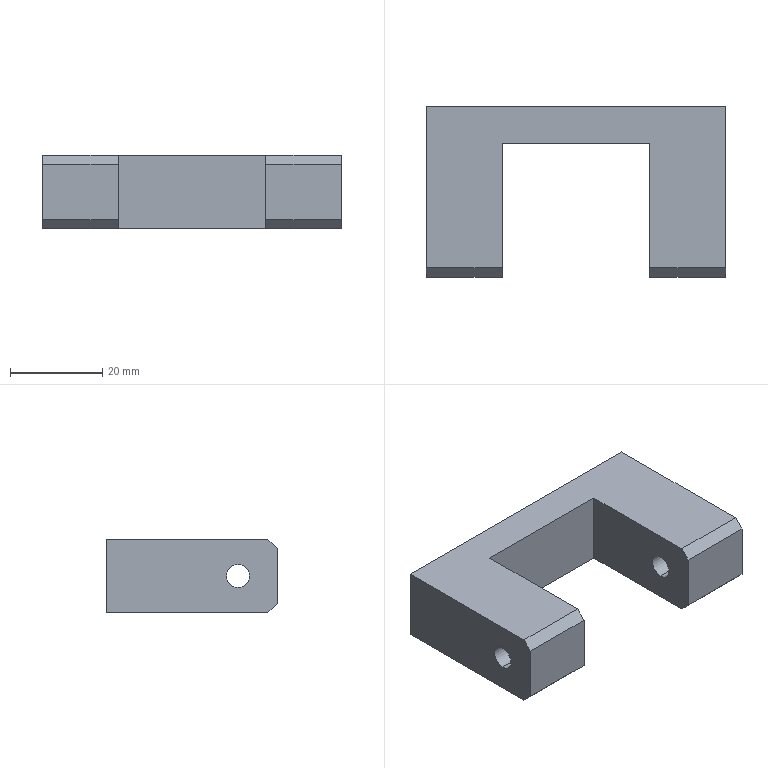Part | SolidWorks | features HoleWzd 3, Chamfer 1, Extrusion 1, ICE 1 | 1 solid | 26 faces | box 65 x 37 x 16 mm | volume 21186 mm3 | plane 14 | cylinder 8 | cone 4 | commonest cylinder face diameters 5 x4 6.8 x4
STEP:
#1=CARTESIAN_POINT('',(-22.5,-3.75,-3.4));
#2=VERTEX_POINT('',#1);
#3=CARTESIAN_POINT('',(-22.5,-3.75,3.4));
#4=VERTEX_POINT('',#3);
#5=CARTESIAN_POINT('',(-22.5,-3.75,0.));
#6=DIRECTION('',(0.,1.,0.));
#7=DIRECTION('',(0.,0.,1.));
#8=AXIS2_PLACEMENT_3D('',#5,#6,#7);
#9=CIRCLE('',#8,3.4);
#10=EDGE_CURVE('',#2,#4,#9,.T.);
#11=ORIENTED_EDGE('',*,*,#10,.F.);
#12=CARTESIAN_POINT('',(-22.5,18.5,-3.4));
#13=VERTEX_POINT('',#12);
#14=CARTESIAN_POINT('',(-22.5,18.5,-3.4));
#15=DIRECTION('',(0.,1.,0.));
#16=VECTOR('',#15,1000.);
#17=LINE('',#14,#16);
#18=EDGE_CURVE('',#2,#13,#17,.T.);
#19=ORIENTED_EDGE('',*,*,#18,.T.);
#20=CARTESIAN_POINT('',(-22.5,18.5,3.4));
#21=VERTEX_POINT('',#20);
#22=CARTESIAN_POINT('',(-22.5,18.5,0.));
#23=DIRECTION('',(0.,1.,0.));
#24=DIRECTION('',(0.,0.,1.));
#25=AXIS2_PLACEMENT_3D('',#22,#23,#24);
#26=CIRCLE('',#25,3.4);
#27=EDGE_CURVE('',#13,#21,#26,.T.);
#28=ORIENTED_EDGE('',*,*,#27,.T.);
#29=CARTESIAN_POINT('',(-22.5,18.5,3.4));
#30=DIRECTION('',(0.,1.,0.));
#31=VECTOR('',#30,1000.);
#32=LINE('',#29,#31);
#33=EDGE_CURVE('',#4,#21,#32,.T.);
#34=ORIENTED_EDGE('',*,*,#33,.F.);
#35=EDGE_LOOP('',(#11,#19,#28,#34));
#36=FACE_OUTER_BOUND('',#35,.T.);
#37=CARTESIAN_POINT('',(-22.5,18.5,0.));
#38=DIRECTION('',(0.,1.,0.));
#39=DIRECTION('',(0.,0.,1.));
#40=AXIS2_PLACEMENT_3D('',#37,#38,#39);
#41=CYLINDRICAL_SURFACE('',#40,3.4);
#42=ADVANCED_FACE('',(#36),#41,.F.);
#43=CARTESIAN_POINT('',(-22.5,-5.793,0.));
#44=VERTEX_POINT('',#43);
#45=CARTESIAN_POINT('',(-22.5,-3.75,3.4));
#46=DIRECTION('',(0.,0.515,0.8572));
#47=VECTOR('',#46,1000.);
#48=LINE('',#45,#47);
#49=EDGE_CURVE('',#44,#4,#48,.T.);
#50=ORIENTED_EDGE('',*,*,#49,.F.);
#51=CARTESIAN_POINT('',(-22.5,-3.75,-3.4));
#52=DIRECTION('',(0.,0.515,-0.8572));
#53=VECTOR('',#52,1000.);
#54=LINE('',#51,#53);
#55=EDGE_CURVE('',#44,#2,#54,.T.);
#56=ORIENTED_EDGE('',*,*,#55,.T.);
#57=ORIENTED_EDGE('',*,*,#10,.T.);
#58=EDGE_LOOP('',(#50,#56,#57));
#59=FACE_OUTER_BOUND('',#58,.T.);
#60=CARTESIAN_POINT('',(-22.5,-3.75,0.));
#61=DIRECTION('',(0.,1.,0.));
#62=DIRECTION('',(0.,0.,1.));
#63=AXIS2_PLACEMENT_3D('',#60,#61,#62);
#64=CONICAL_SURFACE('',#63,3.4,1.03);
#65=ADVANCED_FACE('',(#59),#64,.F.);
#66=CARTESIAN_POINT('',(22.5,-3.75,-3.4));
#67=VERTEX_POINT('',#66);
#68=CARTESIAN_POINT('',(22.5,-3.75,3.4));
#69=VERTEX_POINT('',#68);
#70=CARTESIAN_POINT('',(22.5,-3.75,0.));
#71=DIRECTION('',(0.,1.,0.));
#72=DIRECTION('',(0.,0.,1.));
#73=AXIS2_PLACEMENT_3D('',#70,#71,#72);
#74=CIRCLE('',#73,3.4);
#75=EDGE_CURVE('',#67,#69,#74,.T.);
#76=ORIENTED_EDGE('',*,*,#75,.F.);
#77=CARTESIAN_POINT('',(22.5,18.5,-3.4));
#78=VERTEX_POINT('',#77);
#79=CARTESIAN_POINT('',(22.5,18.5,-3.4));
#80=DIRECTION('',(0.,1.,0.));
#81=VECTOR('',#80,1000.);
#82=LINE('',#79,#81);
#83=EDGE_CURVE('',#67,#78,#82,.T.);
#84=ORIENTED_EDGE('',*,*,#83,.T.);
#85=CARTESIAN_POINT('',(22.5,18.5,3.4));
#86=VERTEX_POINT('',#85);
#87=CARTESIAN_POINT('',(22.5,18.5,0.));
#88=DIRECTION('',(0.,1.,0.));
#89=DIRECTION('',(0.,0.,1.));
#90=AXIS2_PLACEMENT_3D('',#87,#88,#89);
#91=CIRCLE('',#90,3.4);
#92=EDGE_CURVE('',#78,#86,#91,.T.);
#93=ORIENTED_EDGE('',*,*,#92,.T.);
#94=CARTESIAN_POINT('',(22.5,18.5,3.4));
#95=DIRECTION('',(0.,1.,0.));
#96=VECTOR('',#95,1000.);
#97=LINE('',#94,#96);
#98=EDGE_CURVE('',#69,#86,#97,.T.);
#99=ORIENTED_EDGE('',*,*,#98,.F.);
#100=EDGE_LOOP('',(#76,#84,#93,#99));
#101=FACE_OUTER_BOUND('',#100,.T.);
#102=CARTESIAN_POINT('',(22.5,18.5,0.));
#103=DIRECTION('',(0.,1.,0.));
#104=DIRECTION('',(0.,0.,1.));
#105=AXIS2_PLACEMENT_3D('',#102,#103,#104);
#106=CYLINDRICAL_SURFACE('',#105,3.4);
#107=ADVANCED_FACE('',(#101),#106,.F.);
#108=CARTESIAN_POINT('',(22.5,-5.793,0.));
#109=VERTEX_POINT('',#108);
#110=CARTESIAN_POINT('',(22.5,-3.75,3.4));
#111=DIRECTION('',(0.,0.515,0.8572));
#112=VECTOR('',#111,1000.);
#113=LINE('',#110,#112);
#114=EDGE_CURVE('',#109,#69,#113,.T.);
#115=ORIENTED_EDGE('',*,*,#114,.F.);
#116=CARTESIAN_POINT('',(22.5,-3.75,-3.4));
#117=DIRECTION('',(0.,0.515,-0.8572));
#118=VECTOR('',#117,1000.);
#119=LINE('',#116,#118);
#120=EDGE_CURVE('',#109,#67,#119,.T.);
#121=ORIENTED_EDGE('',*,*,#120,.T.);
#122=ORIENTED_EDGE('',*,*,#75,.T.);
#123=EDGE_LOOP('',(#115,#121,#122));
#124=FACE_OUTER_BOUND('',#123,.T.);
#125=CARTESIAN_POINT('',(22.5,-3.75,0.));
#126=DIRECTION('',(0.,1.,0.));
#127=DIRECTION('',(0.,0.,1.));
#128=AXIS2_PLACEMENT_3D('',#125,#126,#127);
#129=CONICAL_SURFACE('',#128,3.4,1.03);
#130=ADVANCED_FACE('',(#124),#129,.F.);
#131=CARTESIAN_POINT('',(-32.5,-10.,2.5));
#132=VERTEX_POINT('',#131);
#133=CARTESIAN_POINT('',(-32.5,-10.,-2.5));
#134=VERTEX_POINT('',#133);
#135=CARTESIAN_POINT('',(-32.5,-10.,0.));
#136=DIRECTION('',(1.,0.,0.));
#137=DIRECTION('',(0.,0.,-1.));
#138=AXIS2_PLACEMENT_3D('',#135,#136,#137);
#139=CIRCLE('',#138,2.5);
#140=EDGE_CURVE('',#132,#134,#139,.T.);
#141=ORIENTED_EDGE('',*,*,#140,.F.);
#142=CARTESIAN_POINT('',(-16.,-10.,2.5));
#143=VERTEX_POINT('',#142);
#144=CARTESIAN_POINT('',(32.5,-10.,2.5));
#145=DIRECTION('',(1.,0.,0.));
#146=VECTOR('',#145,1000.);
#147=LINE('',#144,#146);
#148=EDGE_CURVE('',#132,#143,#147,.T.);
#149=ORIENTED_EDGE('',*,*,#148,.T.);
#150=CARTESIAN_POINT('',(-16.,-10.,-2.5));
#151=VERTEX_POINT('',#150);
#152=CARTESIAN_POINT('',(-16.,-10.,0.));
#153=DIRECTION('',(-1.,0.,0.));
#154=DIRECTION('',(0.,-1.,0.));
#155=AXIS2_PLACEMENT_3D('',#152,#153,#154);
#156=CIRCLE('',#155,2.5);
#157=EDGE_CURVE('',#151,#143,#156,.T.);
#158=ORIENTED_EDGE('',*,*,#157,.F.);
#159=CARTESIAN_POINT('',(32.5,-10.,-2.5));
#160=DIRECTION('',(1.,0.,0.));
#161=VECTOR('',#160,1000.);
#162=LINE('',#159,#161);
#163=EDGE_CURVE('',#134,#151,#162,.T.);
#164=ORIENTED_EDGE('',*,*,#163,.F.);
#165=EDGE_LOOP('',(#141,#149,#158,#164));
#166=FACE_OUTER_BOUND('',#165,.T.);
#167=CARTESIAN_POINT('',(32.5,-10.,0.));
#168=DIRECTION('',(1.,0.,0.));
#169=DIRECTION('',(0.,0.,-1.));
#170=AXIS2_PLACEMENT_3D('',#167,#168,#169);
#171=CYLINDRICAL_SURFACE('',#170,2.5);
#172=ADVANCED_FACE('',(#166),#171,.F.);
#173=CARTESIAN_POINT('',(16.,-10.,2.5));
#174=VERTEX_POINT('',#173);
#175=CARTESIAN_POINT('',(16.,-10.,-2.5));
#176=VERTEX_POINT('',#175);
#177=CARTESIAN_POINT('',(16.,-10.,0.));
#178=DIRECTION('',(1.,0.,0.));
#179=DIRECTION('',(0.,1.,0.));
#180=AXIS2_PLACEMENT_3D('',#177,#178,#179);
#181=CIRCLE('',#180,2.5);
#182=EDGE_CURVE('',#174,#176,#181,.T.);
#183=ORIENTED_EDGE('',*,*,#182,.F.);
#184=CARTESIAN_POINT('',(32.5,-10.,2.5));
#185=VERTEX_POINT('',#184);
#186=CARTESIAN_POINT('',(32.5,-10.,2.5));
#187=DIRECTION('',(1.,0.,0.));
#188=VECTOR('',#187,1000.);
#189=LINE('',#186,#188);
#190=EDGE_CURVE('',#174,#185,#189,.T.);
#191=ORIENTED_EDGE('',*,*,#190,.T.);
#192=CARTESIAN_POINT('',(32.5,-10.,-2.5));
#193=VERTEX_POINT('',#192);
#194=CARTESIAN_POINT('',(32.5,-10.,0.));
#195=DIRECTION('',(1.,0.,0.));
#196=DIRECTION('',(0.,0.,-1.));
#197=AXIS2_PLACEMENT_3D('',#194,#195,#196);
#198=CIRCLE('',#197,2.5);
#199=EDGE_CURVE('',#185,#193,#198,.T.);
#200=ORIENTED_EDGE('',*,*,#199,.T.);
#201=CARTESIAN_POINT('',(32.5,-10.,-2.5));
#202=DIRECTION('',(1.,0.,0.));
#203=VECTOR('',#202,1000.);
#204=LINE('',#201,#203);
#205=EDGE_CURVE('',#176,#193,#204,.T.);
#206=ORIENTED_EDGE('',*,*,#205,.F.);
#207=EDGE_LOOP('',(#183,#191,#200,#206));
#208=FACE_OUTER_BOUND('',#207,.T.);
#209=CARTESIAN_POINT('',(32.5,-10.,0.));
#210=DIRECTION('',(1.,0.,0.));
#211=DIRECTION('',(0.,0.,-1.));
#212=AXIS2_PLACEMENT_3D('',#209,#210,#211);
#213=CYLINDRICAL_SURFACE('',#212,2.5);
#214=ADVANCED_FACE('',(#208),#213,.F.);
#215=CARTESIAN_POINT('',(-32.5,-18.5,6.));
#216=VERTEX_POINT('',#215);
#217=CARTESIAN_POINT('',(-32.5,-18.5,-6.));
#218=VERTEX_POINT('',#217);
#219=CARTESIAN_POINT('',(-32.5,-18.5,8.));
#220=DIRECTION('',(0.,0.,-1.));
#221=VECTOR('',#220,1000.);
#222=LINE('',#219,#221);
#223=EDGE_CURVE('',#216,#218,#222,.T.);
#224=ORIENTED_EDGE('',*,*,#223,.T.);
#225=CARTESIAN_POINT('',(-16.,-18.5,-6.));
#226=VERTEX_POINT('',#225);
#227=CARTESIAN_POINT('',(-32.5,-18.5,-6.));
#228=DIRECTION('',(1.,0.,0.));
#229=VECTOR('',#228,1000.);
#230=LINE('',#227,#229);
#231=EDGE_CURVE('',#218,#226,#230,.T.);
#232=ORIENTED_EDGE('',*,*,#231,.T.);
#233=CARTESIAN_POINT('',(-16.,-18.5,6.));
#234=VERTEX_POINT('',#233);
#235=CARTESIAN_POINT('',(-16.,-18.5,-8.));
#236=DIRECTION('',(0.,0.,1.));
#237=VECTOR('',#236,1000.);
#238=LINE('',#235,#237);
#239=EDGE_CURVE('',#226,#234,#238,.T.);
#240=ORIENTED_EDGE('',*,*,#239,.T.);
#241=CARTESIAN_POINT('',(-32.5,-18.5,6.));
#242=DIRECTION('',(-1.,0.,0.));
#243=VECTOR('',#242,1000.);
#244=LINE('',#241,#243);
#245=EDGE_CURVE('',#234,#216,#244,.T.);
#246=ORIENTED_EDGE('',*,*,#245,.T.);
#247=EDGE_LOOP('',(#224,#232,#240,#246));
#248=FACE_OUTER_BOUND('',#247,.T.);
#249=CARTESIAN_POINT('',(-32.5,-18.5,8.));
#250=DIRECTION('',(0.,1.,0.));
#251=DIRECTION('',(0.,0.,1.));
#252=AXIS2_PLACEMENT_3D('',#249,#250,#251);
#253=PLANE('',#252);
#254=ADVANCED_FACE('',(#248),#253,.F.);
#255=CARTESIAN_POINT('',(-32.5,-10.,0.));
#256=DIRECTION('',(1.,0.,0.));
#257=DIRECTION('',(0.,0.,-1.));
#258=AXIS2_PLACEMENT_3D('',#255,#256,#257);
#259=CIRCLE('',#258,2.5);
#260=EDGE_CURVE('',#134,#132,#259,.T.);
#261=ORIENTED_EDGE('',*,*,#260,.T.);
#262=ORIENTED_EDGE('',*,*,#140,.T.);
#263=EDGE_LOOP('',(#261,#262));
#264=FACE_BOUND('',#263,.T.);
#265=CARTESIAN_POINT('',(-32.5,18.5,-8.));
#266=VERTEX_POINT('',#265);
#267=CARTESIAN_POINT('',(-32.5,-16.5,-8.));
#268=VERTEX_POINT('',#267);
#269=CARTESIAN_POINT('',(-32.5,18.5,-8.));
#270=DIRECTION('',(0.,-1.,0.));
#271=VECTOR('',#270,1000.);
#272=LINE('',#269,#271);
#273=EDGE_CURVE('',#266,#268,#272,.T.);
#274=ORIENTED_EDGE('',*,*,#273,.T.);
#275=CARTESIAN_POINT('',(-32.5,-18.5,-6.));
#276=DIRECTION('',(0.,-0.7071,0.7071));
#277=VECTOR('',#276,1000.);
#278=LINE('',#275,#277);
#279=EDGE_CURVE('',#268,#218,#278,.T.);
#280=ORIENTED_EDGE('',*,*,#279,.T.);
#281=ORIENTED_EDGE('',*,*,#223,.F.);
#282=CARTESIAN_POINT('',(-32.5,-16.5,8.));
#283=VERTEX_POINT('',#282);
#284=CARTESIAN_POINT('',(-32.5,-16.5,8.));
#285=DIRECTION('',(0.,0.7071,0.7071));
#286=VECTOR('',#285,1000.);
#287=LINE('',#284,#286);
#288=EDGE_CURVE('',#216,#283,#287,.T.);
#289=ORIENTED_EDGE('',*,*,#288,.T.);
#290=CARTESIAN_POINT('',(-32.5,18.5,8.));
#291=VERTEX_POINT('',#290);
#292=CARTESIAN_POINT('',(-32.5,18.5,8.));
#293=DIRECTION('',(0.,-1.,0.));
#294=VECTOR('',#293,1000.);
#295=LINE('',#292,#294);
#296=EDGE_CURVE('',#291,#283,#295,.T.);
#297=ORIENTED_EDGE('',*,*,#296,.F.);
#298=CARTESIAN_POINT('',(-32.5,18.5,8.));
#299=DIRECTION('',(0.,0.,-1.));
#300=VECTOR('',#299,1000.);
#301=LINE('',#298,#300);
#302=EDGE_CURVE('',#291,#266,#301,.T.);
#303=ORIENTED_EDGE('',*,*,#302,.T.);
#304=EDGE_LOOP('',(#274,#280,#281,#289,#297,#303));
#305=FACE_OUTER_BOUND('',#304,.T.);
#306=CARTESIAN_POINT('',(-32.5,18.5,8.));
#307=DIRECTION('',(1.,0.,0.));
#308=DIRECTION('',(0.,0.,-1.));
#309=AXIS2_PLACEMENT_3D('',#306,#307,#308);
#310=PLANE('',#309);
#311=ADVANCED_FACE('',(#264,#305),#310,.F.);
#312=CARTESIAN_POINT('',(16.,-18.5,-6.));
#313=VERTEX_POINT('',#312);
#314=CARTESIAN_POINT('',(16.,-18.5,6.));
#315=VERTEX_POINT('',#314);
#316=CARTESIAN_POINT('',(16.,-18.5,-8.));
#317=DIRECTION('',(0.,0.,1.));
#318=VECTOR('',#317,1000.);
#319=LINE('',#316,#318);
#320=EDGE_CURVE('',#313,#315,#319,.T.);
#321=ORIENTED_EDGE('',*,*,#320,.F.);
#322=CARTESIAN_POINT('',(32.5,-18.5,-6.));
#323=VERTEX_POINT('',#322);
#324=CARTESIAN_POINT('',(-32.5,-18.5,-6.));
#325=DIRECTION('',(1.,0.,0.));
#326=VECTOR('',#325,1000.);
#327=LINE('',#324,#326);
#328=EDGE_CURVE('',#313,#323,#327,.T.);
#329=ORIENTED_EDGE('',*,*,#328,.T.);
#330=CARTESIAN_POINT('',(32.5,-18.5,6.));
#331=VERTEX_POINT('',#330);
#332=CARTESIAN_POINT('',(32.5,-18.5,8.));
#333=DIRECTION('',(0.,0.,-1.));
#334=VECTOR('',#333,1000.);
#335=LINE('',#332,#334);
#336=EDGE_CURVE('',#331,#323,#335,.T.);
#337=ORIENTED_EDGE('',*,*,#336,.F.);
#338=CARTESIAN_POINT('',(16.,-18.5,6.));
#339=DIRECTION('',(-1.,0.,0.));
#340=VECTOR('',#339,1000.);
#341=LINE('',#338,#340);
#342=EDGE_CURVE('',#331,#315,#341,.T.);
#343=ORIENTED_EDGE('',*,*,#342,.T.);
#344=EDGE_LOOP('',(#321,#329,#337,#343));
#345=FACE_OUTER_BOUND('',#344,.T.);
#346=CARTESIAN_POINT('',(-32.5,-18.5,8.));
#347=DIRECTION('',(0.,1.,0.));
#348=DIRECTION('',(0.,0.,1.));
#349=AXIS2_PLACEMENT_3D('',#346,#347,#348);
#350=PLANE('',#349);
#351=ADVANCED_FACE('',(#345),#350,.F.);
#352=CARTESIAN_POINT('',(32.5,-10.,0.));
#353=DIRECTION('',(1.,0.,0.));
#354=DIRECTION('',(0.,0.,-1.));
#355=AXIS2_PLACEMENT_3D('',#352,#353,#354);
#356=CIRCLE('',#355,2.5);
#357=EDGE_CURVE('',#193,#185,#356,.T.);
#358=ORIENTED_EDGE('',*,*,#357,.F.);
#359=ORIENTED_EDGE('',*,*,#199,.F.);
#360=EDGE_LOOP('',(#358,#359));
#361=FACE_BOUND('',#360,.T.);
#362=ORIENTED_EDGE('',*,*,#336,.T.);
#363=CARTESIAN_POINT('',(32.5,-16.5,-8.));
#364=VERTEX_POINT('',#363);
#365=CARTESIAN_POINT('',(32.5,-18.5,-6.));
#366=DIRECTION('',(0.,0.7071,-0.7071));
#367=VECTOR('',#366,1000.);
#368=LINE('',#365,#367);
#369=EDGE_CURVE('',#323,#364,#368,.T.);
#370=ORIENTED_EDGE('',*,*,#369,.T.);
#371=CARTESIAN_POINT('',(32.5,18.5,-8.));
#372=VERTEX_POINT('',#371);
#373=CARTESIAN_POINT('',(32.5,18.5,-8.));
#374=DIRECTION('',(0.,1.,0.));
#375=VECTOR('',#374,1000.);
#376=LINE('',#373,#375);
#377=EDGE_CURVE('',#364,#372,#376,.T.);
#378=ORIENTED_EDGE('',*,*,#377,.T.);
#379=CARTESIAN_POINT('',(32.5,18.5,8.));
#380=VERTEX_POINT('',#379);
#381=CARTESIAN_POINT('',(32.5,18.5,8.));
#382=DIRECTION('',(0.,0.,-1.));
#383=VECTOR('',#382,1000.);
#384=LINE('',#381,#383);
#385=EDGE_CURVE('',#380,#372,#384,.T.);
#386=ORIENTED_EDGE('',*,*,#385,.F.);
#387=CARTESIAN_POINT('',(32.5,-16.5,8.));
#388=VERTEX_POINT('',#387);
#389=CARTESIAN_POINT('',(32.5,18.5,8.));
#390=DIRECTION('',(0.,1.,0.));
#391=VECTOR('',#390,1000.);
#392=LINE('',#389,#391);
#393=EDGE_CURVE('',#388,#380,#392,.T.);
#394=ORIENTED_EDGE('',*,*,#393,.F.);
#395=CARTESIAN_POINT('',(32.5,-16.5,8.));
#396=DIRECTION('',(0.,-0.7071,-0.7071));
#397=VECTOR('',#396,1000.);
#398=LINE('',#395,#397);
#399=EDGE_CURVE('',#388,#331,#398,.T.);
#400=ORIENTED_EDGE('',*,*,#399,.T.);
#401=EDGE_LOOP('',(#362,#370,#378,#386,#394,#400));
#402=FACE_OUTER_BOUND('',#401,.T.);
#403=CARTESIAN_POINT('',(32.5,18.5,8.));
#404=DIRECTION('',(-1.,0.,0.));
#405=DIRECTION('',(0.,0.,1.));
#406=AXIS2_PLACEMENT_3D('',#403,#404,#405);
#407=PLANE('',#406);
#408=ADVANCED_FACE('',(#361,#402),#407,.F.);
#409=CARTESIAN_POINT('',(-22.5,18.5,0.));
#410=DIRECTION('',(0.,1.,0.));
#411=DIRECTION('',(0.,0.,1.));
#412=AXIS2_PLACEMENT_3D('',#409,#410,#411);
#413=CIRCLE('',#412,3.4);
#414=EDGE_CURVE('',#21,#13,#413,.T.);
#415=ORIENTED_EDGE('',*,*,#414,.F.);
#416=ORIENTED_EDGE('',*,*,#27,.F.);
#417=EDGE_LOOP('',(#415,#416));
#418=FACE_BOUND('',#417,.T.);
#419=CARTESIAN_POINT('',(22.5,18.5,0.));
#420=DIRECTION('',(0.,1.,0.));
#421=DIRECTION('',(0.,0.,1.));
#422=AXIS2_PLACEMENT_3D('',#419,#420,#421);
#423=CIRCLE('',#422,3.4);
#424=EDGE_CURVE('',#86,#78,#423,.T.);
#425=ORIENTED_EDGE('',*,*,#424,.F.);
#426=ORIENTED_EDGE('',*,*,#92,.F.);
#427=EDGE_LOOP('',(#425,#426));
#428=FACE_BOUND('',#427,.T.);
#429=CARTESIAN_POINT('',(-32.5,18.5,-8.));
#430=DIRECTION('',(-1.,0.,0.));
#431=VECTOR('',#430,1000.);
#432=LINE('',#429,#431);
#433=EDGE_CURVE('',#372,#266,#432,.T.);
#434=ORIENTED_EDGE('',*,*,#433,.T.);
#435=ORIENTED_EDGE('',*,*,#302,.F.);
#436=CARTESIAN_POINT('',(-32.5,18.5,8.));
#437=DIRECTION('',(-1.,0.,0.));
#438=VECTOR('',#437,1000.);
#439=LINE('',#436,#438);
#440=EDGE_CURVE('',#380,#291,#439,.T.);
#441=ORIENTED_EDGE('',*,*,#440,.F.);
#442=ORIENTED_EDGE('',*,*,#385,.T.);
#443=EDGE_LOOP('',(#434,#435,#441,#442));
#444=FACE_OUTER_BOUND('',#443,.T.);
#445=CARTESIAN_POINT('',(-32.5,18.5,8.));
#446=DIRECTION('',(0.,-1.,0.));
#447=DIRECTION('',(0.,0.,-1.));
#448=AXIS2_PLACEMENT_3D('',#445,#446,#447);
#449=PLANE('',#448);
#450=ADVANCED_FACE('',(#418,#428,#444),#449,.F.);
#451=ORIENTED_EDGE('',*,*,#296,.T.);
#452=CARTESIAN_POINT('',(-16.,-16.5,8.));
#453=VERTEX_POINT('',#452);
#454=CARTESIAN_POINT('',(-16.,-16.5,8.));
#455=DIRECTION('',(1.,0.,0.));
#456=VECTOR('',#455,1000.);
#457=LINE('',#454,#456);
#458=EDGE_CURVE('',#283,#453,#457,.T.);
#459=ORIENTED_EDGE('',*,*,#458,.T.);
#460=CARTESIAN_POINT('',(-16.,10.5,8.));
#461=VERTEX_POINT('',#460);
#462=CARTESIAN_POINT('',(-16.,-18.5,8.));
#463=DIRECTION('',(0.,-1.,0.));
#464=VECTOR('',#463,1000.);
#465=LINE('',#462,#464);
#466=EDGE_CURVE('',#461,#453,#465,.T.);
#467=ORIENTED_EDGE('',*,*,#466,.F.);
#468=CARTESIAN_POINT('',(16.,10.5,8.));
#469=VERTEX_POINT('',#468);
#470=CARTESIAN_POINT('',(-16.,10.5,8.));
#471=DIRECTION('',(-1.,0.,0.));
#472=VECTOR('',#471,1000.);
#473=LINE('',#470,#472);
#474=EDGE_CURVE('',#469,#461,#473,.T.);
#475=ORIENTED_EDGE('',*,*,#474,.F.);
#476=CARTESIAN_POINT('',(16.,-16.5,8.));
#477=VERTEX_POINT('',#476);
#478=CARTESIAN_POINT('',(16.,-18.5,8.));
#479=DIRECTION('',(0.,1.,0.));
#480=VECTOR('',#479,1000.);
#481=LINE('',#478,#480);
#482=EDGE_CURVE('',#477,#469,#481,.T.);
#483=ORIENTED_EDGE('',*,*,#482,.F.);
#484=CARTESIAN_POINT('',(32.5,-16.5,8.));
#485=DIRECTION('',(1.,0.,0.));
#486=VECTOR('',#485,1000.);
#487=LINE('',#484,#486);
#488=EDGE_CURVE('',#477,#388,#487,.T.);
#489=ORIENTED_EDGE('',*,*,#488,.T.);
#490=ORIENTED_EDGE('',*,*,#393,.T.);
#491=ORIENTED_EDGE('',*,*,#440,.T.);
#492=EDGE_LOOP('',(#451,#459,#467,#475,#483,#489,#490,#491));
#493=FACE_OUTER_BOUND('',#492,.T.);
#494=CARTESIAN_POINT('',(0.,0.,8.));
#495=DIRECTION('',(0.,0.,1.));
#496=DIRECTION('',(1.,0.,0.));
#497=AXIS2_PLACEMENT_3D('',#494,#495,#496);
#498=PLANE('',#497);
#499=ADVANCED_FACE('',(#493),#498,.T.);
#500=CARTESIAN_POINT('',(-16.,10.5,-8.));
#501=VERTEX_POINT('',#500);
#502=CARTESIAN_POINT('',(-16.,-16.5,-8.));
#503=VERTEX_POINT('',#502);
#504=CARTESIAN_POINT('',(-16.,-18.5,-8.));
#505=DIRECTION('',(0.,-1.,0.));
#506=VECTOR('',#505,1000.);
#507=LINE('',#504,#506);
#508=EDGE_CURVE('',#501,#503,#507,.T.);
#509=ORIENTED_EDGE('',*,*,#508,.T.);
#510=CARTESIAN_POINT('',(0.,-16.5,-8.));
#511=DIRECTION('',(-1.,0.,0.));
#512=VECTOR('',#511,1000.);
#513=LINE('',#510,#512);
#514=EDGE_CURVE('',#503,#268,#513,.T.);
#515=ORIENTED_EDGE('',*,*,#514,.T.);
#516=ORIENTED_EDGE('',*,*,#273,.F.);
#517=ORIENTED_EDGE('',*,*,#433,.F.);
#518=ORIENTED_EDGE('',*,*,#377,.F.);
#519=CARTESIAN_POINT('',(16.,-16.5,-8.));
#520=VERTEX_POINT('',#519);
#521=CARTESIAN_POINT('',(0.,-16.5,-8.));
#522=DIRECTION('',(-1.,0.,0.));
#523=VECTOR('',#522,1000.);
#524=LINE('',#521,#523);
#525=EDGE_CURVE('',#364,#520,#524,.T.);
#526=ORIENTED_EDGE('',*,*,#525,.T.);
#527=CARTESIAN_POINT('',(16.,10.5,-8.));
#528=VERTEX_POINT('',#527);
#529=CARTESIAN_POINT('',(16.,-18.5,-8.));
#530=DIRECTION('',(0.,1.,0.));
#531=VECTOR('',#530,1000.);
#532=LINE('',#529,#531);
#533=EDGE_CURVE('',#520,#528,#532,.T.);
#534=ORIENTED_EDGE('',*,*,#533,.T.);
#535=CARTESIAN_POINT('',(-16.,10.5,-8.));
#536=DIRECTION('',(-1.,0.,0.));
#537=VECTOR('',#536,1000.);
#538=LINE('',#535,#537);
#539=EDGE_CURVE('',#528,#501,#538,.T.);
#540=ORIENTED_EDGE('',*,*,#539,.T.);
#541=EDGE_LOOP('',(#509,#515,#516,#517,#518,#526,#534,#540));
#542=FACE_OUTER_BOUND('',#541,.T.);
#543=CARTESIAN_POINT('',(0.,0.,-8.));
#544=DIRECTION('',(0.,0.,1.));
#545=DIRECTION('',(1.,0.,0.));
#546=AXIS2_PLACEMENT_3D('',#543,#544,#545);
#547=PLANE('',#546);
#548=ADVANCED_FACE('',(#542),#547,.F.);
#549=ORIENTED_EDGE('',*,*,#157,.T.);
#550=CARTESIAN_POINT('',(-16.,-10.,0.));
#551=DIRECTION('',(-1.,0.,0.));
#552=DIRECTION('',(0.,-1.,0.));
#553=AXIS2_PLACEMENT_3D('',#550,#551,#552);
#554=CIRCLE('',#553,2.5);
#555=EDGE_CURVE('',#143,#151,#554,.T.);
#556=ORIENTED_EDGE('',*,*,#555,.T.);
#557=EDGE_LOOP('',(#549,#556));
#558=FACE_BOUND('',#557,.T.);
#559=ORIENTED_EDGE('',*,*,#239,.F.);
#560=CARTESIAN_POINT('',(-16.,-18.5,-6.));
#561=DIRECTION('',(0.,0.7071,-0.7071));
#562=VECTOR('',#561,1000.);
#563=LINE('',#560,#562);
#564=EDGE_CURVE('',#226,#503,#563,.T.);
#565=ORIENTED_EDGE('',*,*,#564,.T.);
#566=ORIENTED_EDGE('',*,*,#508,.F.);
#567=CARTESIAN_POINT('',(-16.,10.5,-8.));
#568=DIRECTION('',(0.,0.,1.));
#569=VECTOR('',#568,1000.);
#570=LINE('',#567,#569);
#571=EDGE_CURVE('',#501,#461,#570,.T.);
#572=ORIENTED_EDGE('',*,*,#571,.T.);
#573=ORIENTED_EDGE('',*,*,#466,.T.);
#574=CARTESIAN_POINT('',(-16.,-16.5,8.));
#575=DIRECTION('',(0.,-0.7071,-0.7071));
#576=VECTOR('',#575,1000.);
#577=LINE('',#574,#576);
#578=EDGE_CURVE('',#453,#234,#577,.T.);
#579=ORIENTED_EDGE('',*,*,#578,.T.);
#580=EDGE_LOOP('',(#559,#565,#566,#572,#573,#579));
#581=FACE_OUTER_BOUND('',#580,.T.);
#582=CARTESIAN_POINT('',(-16.,-18.5,-8.));
#583=DIRECTION('',(-1.,0.,0.));
#584=DIRECTION('',(0.,-1.,0.));
#585=AXIS2_PLACEMENT_3D('',#582,#583,#584);
#586=PLANE('',#585);
#587=ADVANCED_FACE('',(#558,#581),#586,.F.);
#588=ORIENTED_EDGE('',*,*,#474,.T.);
#589=ORIENTED_EDGE('',*,*,#571,.F.);
#590=ORIENTED_EDGE('',*,*,#539,.F.);
#591=CARTESIAN_POINT('',(16.,10.5,-8.));
#592=DIRECTION('',(0.,0.,1.));
#593=VECTOR('',#592,1000.);
#594=LINE('',#591,#593);
#595=EDGE_CURVE('',#528,#469,#594,.T.);
#596=ORIENTED_EDGE('',*,*,#595,.T.);
#597=EDGE_LOOP('',(#588,#589,#590,#596));
#598=FACE_OUTER_BOUND('',#597,.T.);
#599=CARTESIAN_POINT('',(-16.,10.5,-8.));
#600=DIRECTION('',(0.,1.,0.));
#601=DIRECTION('',(-1.,0.,0.));
#602=AXIS2_PLACEMENT_3D('',#599,#600,#601);
#603=PLANE('',#602);
#604=ADVANCED_FACE('',(#598),#603,.F.);
#605=CARTESIAN_POINT('',(16.,-10.,0.));
#606=DIRECTION('',(1.,0.,0.));
#607=DIRECTION('',(0.,1.,0.));
#608=AXIS2_PLACEMENT_3D('',#605,#606,#607);
#609=CIRCLE('',#608,2.5);
#610=EDGE_CURVE('',#176,#174,#609,.T.);
#611=ORIENTED_EDGE('',*,*,#610,.T.);
#612=ORIENTED_EDGE('',*,*,#182,.T.);
#613=EDGE_LOOP('',(#611,#612));
#614=FACE_BOUND('',#613,.T.);
#615=ORIENTED_EDGE('',*,*,#533,.F.);
#616=CARTESIAN_POINT('',(16.,-18.5,-6.));
#617=DIRECTION('',(0.,-0.7071,0.7071));
#618=VECTOR('',#617,1000.);
#619=LINE('',#616,#618);
#620=EDGE_CURVE('',#520,#313,#619,.T.);
#621=ORIENTED_EDGE('',*,*,#620,.T.);
#622=ORIENTED_EDGE('',*,*,#320,.T.);
#623=CARTESIAN_POINT('',(16.,-16.5,8.));
#624=DIRECTION('',(0.,0.7071,0.7071));
#625=VECTOR('',#624,1000.);
#626=LINE('',#623,#625);
#627=EDGE_CURVE('',#315,#477,#626,.T.);
#628=ORIENTED_EDGE('',*,*,#627,.T.);
#629=ORIENTED_EDGE('',*,*,#482,.T.);
#630=ORIENTED_EDGE('',*,*,#595,.F.);
#631=EDGE_LOOP('',(#615,#621,#622,#628,#629,#630));
#632=FACE_OUTER_BOUND('',#631,.T.);
#633=CARTESIAN_POINT('',(16.,-18.5,-8.));
#634=DIRECTION('',(1.,0.,0.));
#635=DIRECTION('',(0.,1.,0.));
#636=AXIS2_PLACEMENT_3D('',#633,#634,#635);
#637=PLANE('',#636);
#638=ADVANCED_FACE('',(#614,#632),#637,.F.);
#639=ORIENTED_EDGE('',*,*,#190,.F.);
#640=ORIENTED_EDGE('',*,*,#610,.F.);
#641=ORIENTED_EDGE('',*,*,#205,.T.);
#642=ORIENTED_EDGE('',*,*,#357,.T.);
#643=EDGE_LOOP('',(#639,#640,#641,#642));
#644=FACE_OUTER_BOUND('',#643,.T.);
#645=CARTESIAN_POINT('',(32.5,-10.,0.));
#646=DIRECTION('',(1.,0.,0.));
#647=DIRECTION('',(0.,0.,-1.));
#648=AXIS2_PLACEMENT_3D('',#645,#646,#647);
#649=CYLINDRICAL_SURFACE('',#648,2.5);
#650=ADVANCED_FACE('',(#644),#649,.F.);
#651=ORIENTED_EDGE('',*,*,#148,.F.);
#652=ORIENTED_EDGE('',*,*,#260,.F.);
#653=ORIENTED_EDGE('',*,*,#163,.T.);
#654=ORIENTED_EDGE('',*,*,#555,.F.);
#655=EDGE_LOOP('',(#651,#652,#653,#654));
#656=FACE_OUTER_BOUND('',#655,.T.);
#657=CARTESIAN_POINT('',(32.5,-10.,0.));
#658=DIRECTION('',(1.,0.,0.));
#659=DIRECTION('',(0.,0.,-1.));
#660=AXIS2_PLACEMENT_3D('',#657,#658,#659);
#661=CYLINDRICAL_SURFACE('',#660,2.5);
#662=ADVANCED_FACE('',(#656),#661,.F.);
#663=ORIENTED_EDGE('',*,*,#120,.F.);
#664=ORIENTED_EDGE('',*,*,#114,.T.);
#665=CARTESIAN_POINT('',(22.5,-3.75,0.));
#666=DIRECTION('',(0.,1.,0.));
#667=DIRECTION('',(0.,0.,1.));
#668=AXIS2_PLACEMENT_3D('',#665,#666,#667);
#669=CIRCLE('',#668,3.4);
#670=EDGE_CURVE('',#69,#67,#669,.T.);
#671=ORIENTED_EDGE('',*,*,#670,.T.);
#672=EDGE_LOOP('',(#663,#664,#671));
#673=FACE_OUTER_BOUND('',#672,.T.);
#674=CARTESIAN_POINT('',(22.5,-3.75,0.));
#675=DIRECTION('',(0.,1.,0.));
#676=DIRECTION('',(0.,0.,1.));
#677=AXIS2_PLACEMENT_3D('',#674,#675,#676);
#678=CONICAL_SURFACE('',#677,3.4,1.03);
#679=ADVANCED_FACE('',(#673),#678,.F.);
#680=ORIENTED_EDGE('',*,*,#83,.F.);
#681=ORIENTED_EDGE('',*,*,#670,.F.);
#682=ORIENTED_EDGE('',*,*,#98,.T.);
#683=ORIENTED_EDGE('',*,*,#424,.T.);
#684=EDGE_LOOP('',(#680,#681,#682,#683));
#685=FACE_OUTER_BOUND('',#684,.T.);
#686=CARTESIAN_POINT('',(22.5,18.5,0.));
#687=DIRECTION('',(0.,1.,0.));
#688=DIRECTION('',(0.,0.,1.));
#689=AXIS2_PLACEMENT_3D('',#686,#687,#688);
#690=CYLINDRICAL_SURFACE('',#689,3.4);
#691=ADVANCED_FACE('',(#685),#690,.F.);
#692=ORIENTED_EDGE('',*,*,#55,.F.);
#693=ORIENTED_EDGE('',*,*,#49,.T.);
#694=CARTESIAN_POINT('',(-22.5,-3.75,0.));
#695=DIRECTION('',(0.,1.,0.));
#696=DIRECTION('',(0.,0.,1.));
#697=AXIS2_PLACEMENT_3D('',#694,#695,#696);
#698=CIRCLE('',#697,3.4);
#699=EDGE_CURVE('',#4,#2,#698,.T.);
#700=ORIENTED_EDGE('',*,*,#699,.T.);
#701=EDGE_LOOP('',(#692,#693,#700));
#702=FACE_OUTER_BOUND('',#701,.T.);
#703=CARTESIAN_POINT('',(-22.5,-3.75,0.));
#704=DIRECTION('',(0.,1.,0.));
#705=DIRECTION('',(0.,0.,1.));
#706=AXIS2_PLACEMENT_3D('',#703,#704,#705);
#707=CONICAL_SURFACE('',#706,3.4,1.03);
#708=ADVANCED_FACE('',(#702),#707,.F.);
#709=ORIENTED_EDGE('',*,*,#18,.F.);
#710=ORIENTED_EDGE('',*,*,#699,.F.);
#711=ORIENTED_EDGE('',*,*,#33,.T.);
#712=ORIENTED_EDGE('',*,*,#414,.T.);
#713=EDGE_LOOP('',(#709,#710,#711,#712));
#714=FACE_OUTER_BOUND('',#713,.T.);
#715=CARTESIAN_POINT('',(-22.5,18.5,0.));
#716=DIRECTION('',(0.,1.,0.));
#717=DIRECTION('',(0.,0.,1.));
#718=AXIS2_PLACEMENT_3D('',#715,#716,#717);
#719=CYLINDRICAL_SURFACE('',#718,3.4);
#720=ADVANCED_FACE('',(#714),#719,.F.);
#721=ORIENTED_EDGE('',*,*,#279,.F.);
#722=ORIENTED_EDGE('',*,*,#514,.F.);
#723=ORIENTED_EDGE('',*,*,#564,.F.);
#724=ORIENTED_EDGE('',*,*,#231,.F.);
#725=EDGE_LOOP('',(#721,#722,#723,#724));
#726=FACE_OUTER_BOUND('',#725,.T.);
#727=CARTESIAN_POINT('',(-32.5,-18.5,-6.));
#728=DIRECTION('',(0.,0.7071,0.7071));
#729=DIRECTION('',(1.,0.,0.));
#730=AXIS2_PLACEMENT_3D('',#727,#728,#729);
#731=PLANE('',#730);
#732=ADVANCED_FACE('',(#726),#731,.F.);
#733=ORIENTED_EDGE('',*,*,#288,.F.);
#734=ORIENTED_EDGE('',*,*,#245,.F.);
#735=ORIENTED_EDGE('',*,*,#578,.F.);
#736=ORIENTED_EDGE('',*,*,#458,.F.);
#737=EDGE_LOOP('',(#733,#734,#735,#736));
#738=FACE_OUTER_BOUND('',#737,.T.);
#739=CARTESIAN_POINT('',(0.,-16.5,8.));
#740=DIRECTION('',(0.,-0.7071,0.7071));
#741=DIRECTION('',(-1.,0.,0.));
#742=AXIS2_PLACEMENT_3D('',#739,#740,#741);
#743=PLANE('',#742);
#744=ADVANCED_FACE('',(#738),#743,.T.);
#745=ORIENTED_EDGE('',*,*,#620,.F.);
#746=ORIENTED_EDGE('',*,*,#525,.F.);
#747=ORIENTED_EDGE('',*,*,#369,.F.);
#748=ORIENTED_EDGE('',*,*,#328,.F.);
#749=EDGE_LOOP('',(#745,#746,#747,#748));
#750=FACE_OUTER_BOUND('',#749,.T.);
#751=CARTESIAN_POINT('',(-32.5,-18.5,-6.));
#752=DIRECTION('',(0.,0.7071,0.7071));
#753=DIRECTION('',(1.,0.,0.));
#754=AXIS2_PLACEMENT_3D('',#751,#752,#753);
#755=PLANE('',#754);
#756=ADVANCED_FACE('',(#750),#755,.F.);
#757=ORIENTED_EDGE('',*,*,#627,.F.);
#758=ORIENTED_EDGE('',*,*,#342,.F.);
#759=ORIENTED_EDGE('',*,*,#399,.F.);
#760=ORIENTED_EDGE('',*,*,#488,.F.);
#761=EDGE_LOOP('',(#757,#758,#759,#760));
#762=FACE_OUTER_BOUND('',#761,.T.);
#763=CARTESIAN_POINT('',(0.,-16.5,8.));
#764=DIRECTION('',(0.,-0.7071,0.7071));
#765=DIRECTION('',(-1.,0.,0.));
#766=AXIS2_PLACEMENT_3D('',#763,#764,#765);
#767=PLANE('',#766);
#768=ADVANCED_FACE('',(#762),#767,.T.);
#769=CLOSED_SHELL('',(#42,#65,#107,#130,#172,#214,#254,#311,#351,#408,#450,#499,#548,#587,#604,#638,#650,#662,#679,#691,#708,#720,#732,#744,#756,#768));
#770=MANIFOLD_SOLID_BREP('',#769);
#771=CARTESIAN_POINT('',(0.,0.,0.));
#772=DIRECTION('',(0.,0.,1.));
#773=DIRECTION('',(1.,0.,0.));
#774=AXIS2_PLACEMENT_3D('',#771,#772,#773);
#775=(LENGTH_UNIT()NAMED_UNIT(*)SI_UNIT(.MILLI.,.METRE.));
#776=UNCERTAINTY_MEASURE_WITH_UNIT(LENGTH_MEASURE(0.00001),#775,'','');
#777=(NAMED_UNIT(*)PLANE_ANGLE_UNIT()SI_UNIT($,.RADIAN.));
#778=(NAMED_UNIT(*)SI_UNIT($,.STERADIAN.)SOLID_ANGLE_UNIT());
#779=(GEOMETRIC_REPRESENTATION_CONTEXT(3)GLOBAL_UNCERTAINTY_ASSIGNED_CONTEXT((#776))GLOBAL_UNIT_ASSIGNED_CONTEXT((#775,#777,#778))REPRESENTATION_CONTEXT('',''));
#780=ADVANCED_BREP_SHAPE_REPRESENTATION('',(#770,#774),#779);